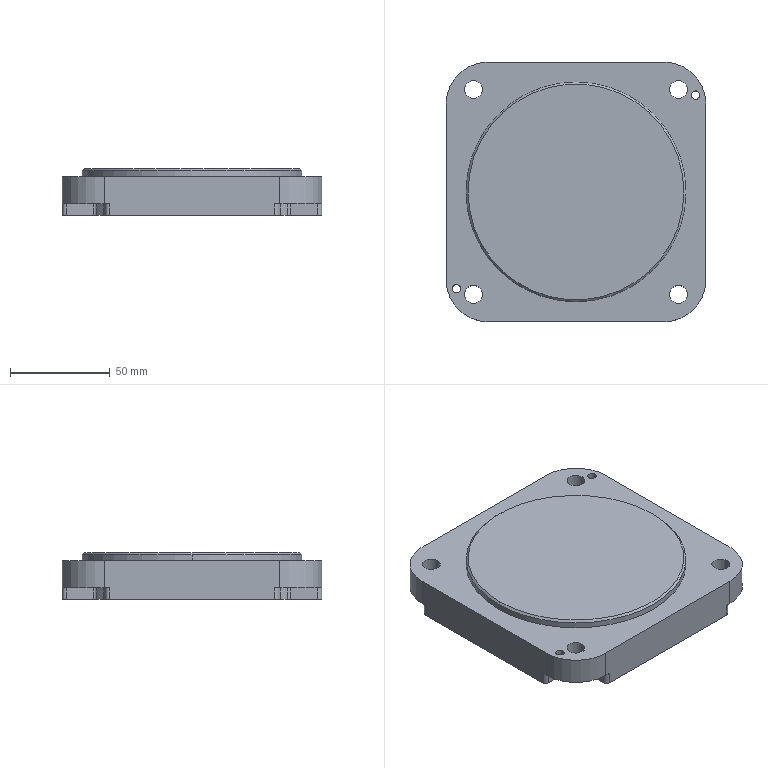Part | STEP file | 31090345--1-SOL000 | 1 solid | 59 faces | box 130 x 130 x 23.5 mm | volume 347799 mm3 | cylinder 38 | plane 19 | cone 2 | commonest cylinder face diameters 4 x16 9 x8 4.2 x4 42 x4 130 x4 110 x2